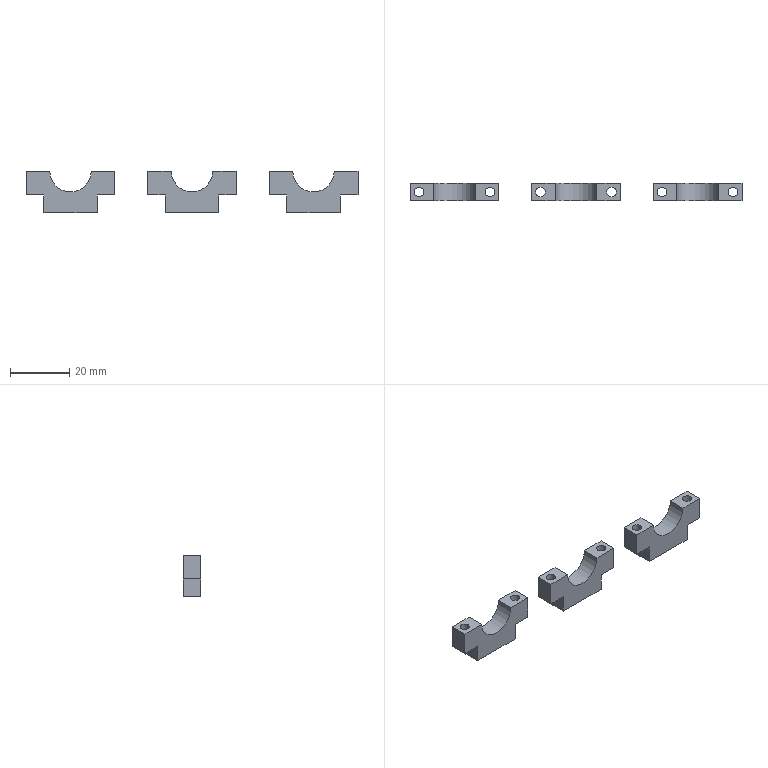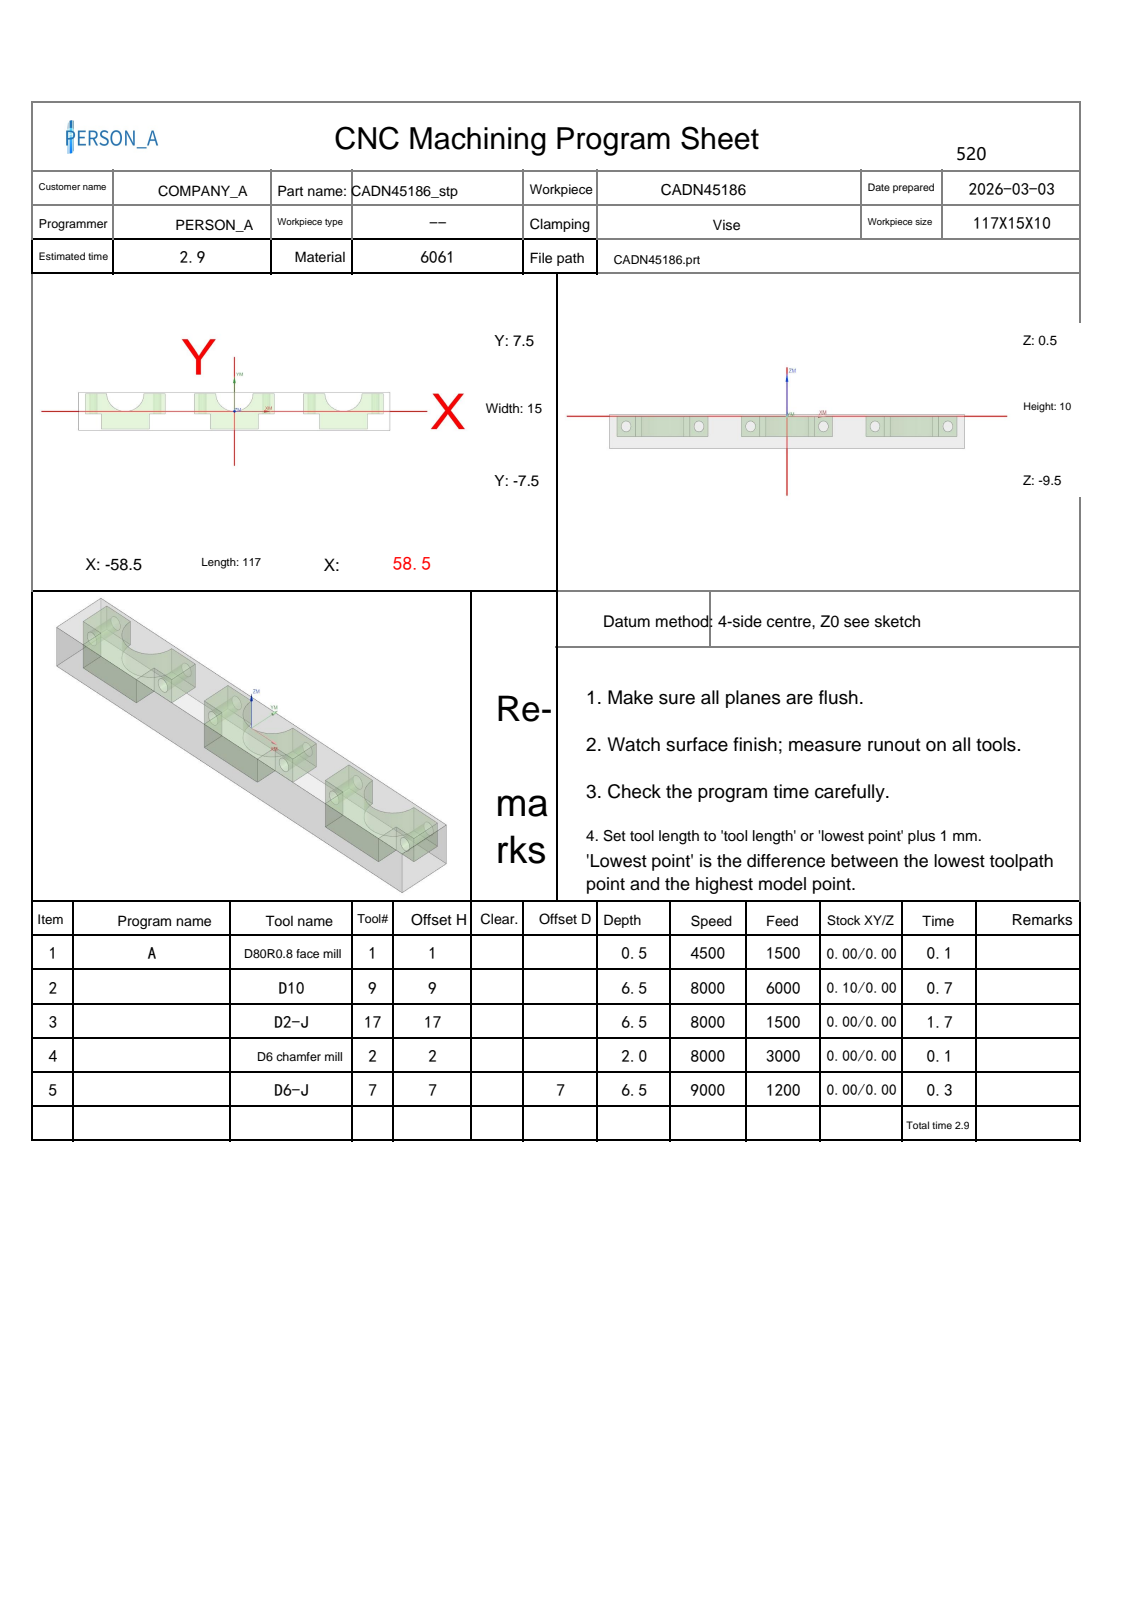NC program | NX | posted by the shop | part box 112 x 6 x 14 mm
Lines 634 to 1728 of 5059:
N3 T17 M06
(D2-J  D=2. R=0. H=17 ce=0.00 di=0.00)
(MAX_Z=50. MIN_Z=-6. Time=1.66M)
G00 G90 G54 X55.15 Y-2.2 M03 S8000
G43 H17 Z50.
M08
Z0.0
G01 X55.149 Y-2.197 Z-.03 F1500.
X55.147 Y-2.19 Z-.058
X55.144 Y-2.179 Z-.082
X55.139 Y-2.165 Z-.104
X55.133 Y-2.148 Z-.123
X55.125 Y-2.13 Z-.14
X55.115 Y-2.11 Z-.154
X55.103 Y-2.09 Z-.166
X55.089 Y-2.07 Z-.176
X55.072 Y-2.052 Z-.184
X55.053 Y-2.035 Z-.19
X55.032 Y-2.021 Z-.195
X55.007 Y-2.01 Z-.198
X54.98 Y-2.003 Z-.199
X54.95 Y-2. Z-.2
X51.
Y-5.95
X51.014 Y-5.964 Z-.201
X51.056 Y-5.953 Z-.202
X51.121 Y-5.919 Z-.205
X51.209 Y-5.864 Z-.209
X51.565 Y-5.599 Z-.225
X51.878 Y-5.345 Z-.239
X52.111 Y-5.146 Z-.249
X52.375 Y-4.909 Z-.262
X52.674 Y-4.632 Z-.276
X52.995 Y-4.322 Z-.292
X53.322 Y-3.995 Z-.308
X53.632 Y-3.674 Z-.324
X53.909 Y-3.375 Z-.338
X54.146 Y-3.111 Z-.351
X54.345 Y-2.878 Z-.361
X54.599 Y-2.565 Z-.375
X54.864 Y-2.209 Z-.391
X54.919 Y-2.121 Z-.395
X54.953 Y-2.056 Z-.398
X54.964 Y-2.014 Z-.399
X54.95 Y-2. Z-.4
X51.
Y-5.95
X51.014 Y-5.964 Z-.401
X51.056 Y-5.953 Z-.402
X51.121 Y-5.919 Z-.405
X51.209 Y-5.864 Z-.409
X51.565 Y-5.599 Z-.425
X51.878 Y-5.345 Z-.439
X52.111 Y-5.146 Z-.449
X52.375 Y-4.909 Z-.462
X52.674 Y-4.632 Z-.476
X52.995 Y-4.322 Z-.492
X53.322 Y-3.995 Z-.508
X53.632 Y-3.674 Z-.524
X53.909 Y-3.375 Z-.538
X54.146 Y-3.111 Z-.551
X54.345 Y-2.878 Z-.561
X54.599 Y-2.565 Z-.575
X54.864 Y-2.209 Z-.591
X54.919 Y-2.121 Z-.595
X54.953 Y-2.056 Z-.598
X54.964 Y-2.014 Z-.599
X54.95 Y-2. Z-.6
X51.
Y-5.95
X51.014 Y-5.964 Z-.601
X51.056 Y-5.953 Z-.602
X51.121 Y-5.919 Z-.605
X51.209 Y-5.864 Z-.609
X51.565 Y-5.599 Z-.625
X51.878 Y-5.345 Z-.639
X52.111 Y-5.146 Z-.649
X52.375 Y-4.909 Z-.662
X52.674 Y-4.632 Z-.676
X52.995 Y-4.322 Z-.692
X53.322 Y-3.995 Z-.708
X53.632 Y-3.674 Z-.724
X53.909 Y-3.375 Z-.738
X54.146 Y-3.111 Z-.751
X54.345 Y-2.878 Z-.761
X54.599 Y-2.565 Z-.775
X54.864 Y-2.209 Z-.791
X54.919 Y-2.121 Z-.795
X54.953 Y-2.056 Z-.798
X54.964 Y-2.014 Z-.799
X54.95 Y-2. Z-.8
X51.
Y-5.95
X51.014 Y-5.964 Z-.801
X51.056 Y-5.953 Z-.802
X51.121 Y-5.919 Z-.805
X51.209 Y-5.864 Z-.809
X51.565 Y-5.599 Z-.825
X51.878 Y-5.345 Z-.839
X52.111 Y-5.146 Z-.849
X52.375 Y-4.909 Z-.862
X52.674 Y-4.632 Z-.876
X52.995 Y-4.322 Z-.892
X53.322 Y-3.995 Z-.908
X53.632 Y-3.674 Z-.924
X53.909 Y-3.375 Z-.938
X54.146 Y-3.111 Z-.951
X54.345 Y-2.878 Z-.961
X54.599 Y-2.565 Z-.975
X54.864 Y-2.209 Z-.991
X54.919 Y-2.121 Z-.995
X54.953 Y-2.056 Z-.998
X54.964 Y-2.014 Z-.999
X54.95 Y-2. Z-1.
X51.
Y-5.95
X51.014 Y-5.964 Z-1.001
X51.056 Y-5.953 Z-1.002
X51.121 Y-5.919 Z-1.005
X51.209 Y-5.864 Z-1.009
X51.565 Y-5.599 Z-1.025
X51.878 Y-5.345 Z-1.039
X52.111 Y-5.146 Z-1.049
X52.375 Y-4.909 Z-1.062
X52.674 Y-4.632 Z-1.076
X52.995 Y-4.322 Z-1.092
X53.322 Y-3.995 Z-1.108
X53.632 Y-3.674 Z-1.124
X53.909 Y-3.375 Z-1.138
X54.146 Y-3.111 Z-1.151
X54.345 Y-2.878 Z-1.161
X54.599 Y-2.565 Z-1.175
X54.864 Y-2.209 Z-1.191
X54.919 Y-2.121 Z-1.195
X54.953 Y-2.056 Z-1.198
X54.964 Y-2.014 Z-1.199
X54.95 Y-2. Z-1.2
X51.
Y-5.95
X51.014 Y-5.964 Z-1.201
X51.056 Y-5.953 Z-1.202
X51.121 Y-5.919 Z-1.205
X51.209 Y-5.864 Z-1.209
X51.565 Y-5.599 Z-1.225
X51.878 Y-5.345 Z-1.239
X52.111 Y-5.146 Z-1.249
X52.375 Y-4.909 Z-1.262
X52.674 Y-4.632 Z-1.276
X52.995 Y-4.322 Z-1.292
X53.322 Y-3.995 Z-1.308
X53.632 Y-3.674 Z-1.324
X53.909 Y-3.375 Z-1.338
X54.146 Y-3.111 Z-1.351
X54.345 Y-2.878 Z-1.361
X54.599 Y-2.565 Z-1.375
X54.864 Y-2.209 Z-1.391
X54.919 Y-2.121 Z-1.395
X54.953 Y-2.056 Z-1.398
X54.964 Y-2.014 Z-1.399
X54.95 Y-2. Z-1.4
X51.
Y-5.95
X51.014 Y-5.964 Z-1.401
X51.056 Y-5.953 Z-1.402
X51.121 Y-5.919 Z-1.405
X51.209 Y-5.864 Z-1.409
X51.565 Y-5.599 Z-1.425
X51.878 Y-5.345 Z-1.439
X52.111 Y-5.146 Z-1.449
X52.375 Y-4.909 Z-1.462
X52.674 Y-4.632 Z-1.476
X52.995 Y-4.322 Z-1.492
X53.322 Y-3.995 Z-1.508
X53.632 Y-3.674 Z-1.524
X53.909 Y-3.375 Z-1.538
X54.146 Y-3.111 Z-1.551
X54.345 Y-2.878 Z-1.561
X54.599 Y-2.565 Z-1.575
X54.864 Y-2.209 Z-1.591
X54.919 Y-2.121 Z-1.595
X54.953 Y-2.056 Z-1.598
X54.964 Y-2.014 Z-1.599
X54.95 Y-2. Z-1.6
X51.
Y-5.95
X51.014 Y-5.964 Z-1.601
X51.056 Y-5.953 Z-1.602
X51.121 Y-5.919 Z-1.605
X51.209 Y-5.864 Z-1.609
X51.565 Y-5.599 Z-1.625
X51.878 Y-5.345 Z-1.639
X52.111 Y-5.146 Z-1.649
X52.375 Y-4.909 Z-1.662
X52.674 Y-4.632 Z-1.676
X52.995 Y-4.322 Z-1.692
X53.322 Y-3.995 Z-1.708
X53.632 Y-3.674 Z-1.724
X53.909 Y-3.375 Z-1.738
X54.146 Y-3.111 Z-1.751
X54.345 Y-2.878 Z-1.761
X54.599 Y-2.565 Z-1.775
X54.864 Y-2.209 Z-1.791
X54.919 Y-2.121 Z-1.795
X54.953 Y-2.056 Z-1.798
X54.964 Y-2.014 Z-1.799
X54.95 Y-2. Z-1.8
X51.
Y-5.95
X51.014 Y-5.964 Z-1.801
X51.056 Y-5.953 Z-1.802
X51.121 Y-5.919 Z-1.805
X51.209 Y-5.864 Z-1.809
X51.565 Y-5.599 Z-1.825
X51.878 Y-5.345 Z-1.839
X52.111 Y-5.146 Z-1.849
X52.375 Y-4.909 Z-1.862
X52.674 Y-4.632 Z-1.876
X52.995 Y-4.322 Z-1.892
X53.322 Y-3.995 Z-1.908
X53.632 Y-3.674 Z-1.924
X53.909 Y-3.375 Z-1.938
X54.146 Y-3.111 Z-1.951
X54.345 Y-2.878 Z-1.961
X54.599 Y-2.565 Z-1.975
X54.864 Y-2.209 Z-1.991
X54.919 Y-2.121 Z-1.995
X54.953 Y-2.056 Z-1.998
X54.964 Y-2.014 Z-1.999
X54.95 Y-2. Z-2.
X51.
Y-5.95
X51.014 Y-5.964 Z-2.001
X51.056 Y-5.953 Z-2.002
X51.121 Y-5.919 Z-2.005
X51.209 Y-5.864 Z-2.009
X51.565 Y-5.599 Z-2.025
X51.878 Y-5.345 Z-2.039
X52.111 Y-5.146 Z-2.049
X52.375 Y-4.909 Z-2.062
X52.674 Y-4.632 Z-2.076
X52.995 Y-4.322 Z-2.092
X53.322 Y-3.995 Z-2.108
X53.632 Y-3.674 Z-2.124
X53.909 Y-3.375 Z-2.138
X54.146 Y-3.111 Z-2.151
X54.345 Y-2.878 Z-2.161
X54.599 Y-2.565 Z-2.175
X54.864 Y-2.209 Z-2.191
X54.919 Y-2.121 Z-2.195
X54.953 Y-2.056 Z-2.198
X54.964 Y-2.014 Z-2.199
X54.95 Y-2. Z-2.2
X51.
Y-5.95
X51.014 Y-5.964 Z-2.201
X51.056 Y-5.953 Z-2.202
X51.121 Y-5.919 Z-2.205
X51.209 Y-5.864 Z-2.209
X51.565 Y-5.599 Z-2.225
X51.878 Y-5.345 Z-2.239
X52.111 Y-5.146 Z-2.249
X52.375 Y-4.909 Z-2.262
X52.674 Y-4.632 Z-2.276
X52.995 Y-4.322 Z-2.292
X53.322 Y-3.995 Z-2.308
X53.632 Y-3.674 Z-2.324
X53.909 Y-3.375 Z-2.338
X54.146 Y-3.111 Z-2.351
X54.345 Y-2.878 Z-2.361
X54.599 Y-2.565 Z-2.375
X54.864 Y-2.209 Z-2.391
X54.919 Y-2.121 Z-2.395
X54.953 Y-2.056 Z-2.398
X54.964 Y-2.014 Z-2.399
X54.95 Y-2. Z-2.4
X51.
Y-5.95
X51.014 Y-5.964 Z-2.401
X51.056 Y-5.953 Z-2.402
X51.121 Y-5.919 Z-2.405
X51.209 Y-5.864 Z-2.409
X51.565 Y-5.599 Z-2.425
X51.878 Y-5.345 Z-2.439
X52.111 Y-5.146 Z-2.449
X52.375 Y-4.909 Z-2.462
X52.674 Y-4.632 Z-2.476
X52.995 Y-4.322 Z-2.492
X53.322 Y-3.995 Z-2.508
X53.632 Y-3.674 Z-2.524
X53.909 Y-3.375 Z-2.538
X54.146 Y-3.111 Z-2.551
X54.345 Y-2.878 Z-2.561
X54.599 Y-2.565 Z-2.575
X54.864 Y-2.209 Z-2.591
X54.919 Y-2.121 Z-2.595
X54.953 Y-2.056 Z-2.598
X54.964 Y-2.014 Z-2.599
X54.95 Y-2. Z-2.6
X51.
Y-5.95
X51.014 Y-5.964 Z-2.601
X51.056 Y-5.953 Z-2.602
X51.121 Y-5.919 Z-2.605
X51.209 Y-5.864 Z-2.609
X51.565 Y-5.599 Z-2.625
X51.878 Y-5.345 Z-2.639
X52.111 Y-5.146 Z-2.649
X52.375 Y-4.909 Z-2.662
X52.674 Y-4.632 Z-2.676
X52.995 Y-4.322 Z-2.692
X53.322 Y-3.995 Z-2.708
X53.632 Y-3.674 Z-2.724
X53.909 Y-3.375 Z-2.738
X54.146 Y-3.111 Z-2.751
X54.345 Y-2.878 Z-2.761
X54.599 Y-2.565 Z-2.775
X54.864 Y-2.209 Z-2.791
X54.919 Y-2.121 Z-2.795
X54.953 Y-2.056 Z-2.798
X54.964 Y-2.014 Z-2.799
X54.95 Y-2. Z-2.8
X51.
Y-5.95
X51.014 Y-5.964 Z-2.801
X51.056 Y-5.953 Z-2.802
X51.121 Y-5.919 Z-2.805
X51.209 Y-5.864 Z-2.809
X51.565 Y-5.599 Z-2.825
X51.878 Y-5.345 Z-2.839
X52.111 Y-5.146 Z-2.849
X52.375 Y-4.909 Z-2.862
X52.674 Y-4.632 Z-2.876
X52.995 Y-4.322 Z-2.892
X53.322 Y-3.995 Z-2.908
X53.632 Y-3.674 Z-2.924
X53.909 Y-3.375 Z-2.938
X54.146 Y-3.111 Z-2.951
X54.345 Y-2.878 Z-2.961
X54.599 Y-2.565 Z-2.975
X54.864 Y-2.209 Z-2.991
X54.919 Y-2.121 Z-2.995
X54.953 Y-2.056 Z-2.998
X54.964 Y-2.014 Z-2.999
X54.95 Y-2. Z-3.
X51.
Y-5.95
X51.014 Y-5.964 Z-3.001
X51.056 Y-5.953 Z-3.002
X51.121 Y-5.919 Z-3.005
X51.209 Y-5.864 Z-3.009
X51.565 Y-5.599 Z-3.025
X51.878 Y-5.345 Z-3.039
X52.111 Y-5.146 Z-3.049
X52.375 Y-4.909 Z-3.062
X52.674 Y-4.632 Z-3.076
X52.995 Y-4.322 Z-3.092
X53.322 Y-3.995 Z-3.108
X53.632 Y-3.674 Z-3.124
X53.909 Y-3.375 Z-3.138
X54.146 Y-3.111 Z-3.151
X54.345 Y-2.878 Z-3.161
X54.599 Y-2.565 Z-3.175
X54.864 Y-2.209 Z-3.191
X54.919 Y-2.121 Z-3.195
X54.953 Y-2.056 Z-3.198
X54.964 Y-2.014 Z-3.199
X54.95 Y-2. Z-3.2
X51.
Y-5.95
X51.014 Y-5.964 Z-3.201
X51.056 Y-5.953 Z-3.202
X51.121 Y-5.919 Z-3.205
X51.209 Y-5.864 Z-3.209
X51.565 Y-5.599 Z-3.225
X51.878 Y-5.345 Z-3.239
X52.111 Y-5.146 Z-3.249
X52.375 Y-4.909 Z-3.262
X52.674 Y-4.632 Z-3.276
X52.995 Y-4.322 Z-3.292
X53.322 Y-3.995 Z-3.308
X53.632 Y-3.674 Z-3.324
X53.909 Y-3.375 Z-3.338
X54.146 Y-3.111 Z-3.351
X54.345 Y-2.878 Z-3.361
X54.599 Y-2.565 Z-3.375
X54.864 Y-2.209 Z-3.391
X54.919 Y-2.121 Z-3.395
X54.953 Y-2.056 Z-3.398
X54.964 Y-2.014 Z-3.399
X54.95 Y-2. Z-3.4
X51.
Y-5.95
X51.014 Y-5.964 Z-3.401
X51.056 Y-5.953 Z-3.402
X51.121 Y-5.919 Z-3.405
X51.209 Y-5.864 Z-3.409
X51.565 Y-5.599 Z-3.425
X51.878 Y-5.345 Z-3.439
X52.111 Y-5.146 Z-3.449
X52.375 Y-4.909 Z-3.462
X52.674 Y-4.632 Z-3.476
X52.995 Y-4.322 Z-3.492
X53.322 Y-3.995 Z-3.508
X53.632 Y-3.674 Z-3.524
X53.909 Y-3.375 Z-3.538
X54.146 Y-3.111 Z-3.551
X54.345 Y-2.878 Z-3.561
X54.599 Y-2.565 Z-3.575
X54.864 Y-2.209 Z-3.591
X54.919 Y-2.121 Z-3.595
X54.953 Y-2.056 Z-3.598
X54.964 Y-2.014 Z-3.599
X54.95 Y-2. Z-3.6
X51.
Y-5.95
X51.014 Y-5.964 Z-3.601
X51.056 Y-5.953 Z-3.602
X51.121 Y-5.919 Z-3.605
X51.209 Y-5.864 Z-3.609
X51.565 Y-5.599 Z-3.625
X51.878 Y-5.345 Z-3.639
X52.111 Y-5.146 Z-3.649
X52.375 Y-4.909 Z-3.662
X52.674 Y-4.632 Z-3.676
X52.995 Y-4.322 Z-3.692
X53.322 Y-3.995 Z-3.708
X53.632 Y-3.674 Z-3.724
X53.909 Y-3.375 Z-3.738
X54.146 Y-3.111 Z-3.751
X54.345 Y-2.878 Z-3.761
X54.599 Y-2.565 Z-3.775
X54.864 Y-2.209 Z-3.791
X54.919 Y-2.121 Z-3.795
X54.953 Y-2.056 Z-3.798
X54.964 Y-2.014 Z-3.799
X54.95 Y-2. Z-3.8
X51.
Y-5.95
X51.014 Y-5.964 Z-3.801
X51.056 Y-5.953 Z-3.802
X51.121 Y-5.919 Z-3.805
X51.209 Y-5.864 Z-3.809
X51.565 Y-5.599 Z-3.825
X51.878 Y-5.345 Z-3.839
X52.111 Y-5.146 Z-3.849
X52.375 Y-4.909 Z-3.862
X52.674 Y-4.632 Z-3.876
X52.995 Y-4.322 Z-3.892
X53.322 Y-3.995 Z-3.908
X53.632 Y-3.674 Z-3.924
X53.909 Y-3.375 Z-3.938
X54.146 Y-3.111 Z-3.951
X54.345 Y-2.878 Z-3.961
X54.599 Y-2.565 Z-3.975
X54.864 Y-2.209 Z-3.991
X54.919 Y-2.121 Z-3.995
X54.953 Y-2.056 Z-3.998
X54.964 Y-2.014 Z-3.999
X54.95 Y-2. Z-4.
X51.
Y-5.95
X51.014 Y-5.964 Z-4.001
X51.056 Y-5.953 Z-4.002
X51.121 Y-5.919 Z-4.005
X51.209 Y-5.864 Z-4.009
X51.565 Y-5.599 Z-4.025
X51.878 Y-5.345 Z-4.039
X52.111 Y-5.146 Z-4.049
X52.375 Y-4.909 Z-4.062
X52.674 Y-4.632 Z-4.076
X52.995 Y-4.322 Z-4.092
X53.322 Y-3.995 Z-4.108
X53.632 Y-3.674 Z-4.124
X53.909 Y-3.375 Z-4.138
X54.146 Y-3.111 Z-4.151
X54.345 Y-2.878 Z-4.161
X54.599 Y-2.565 Z-4.175
X54.864 Y-2.209 Z-4.191
X54.919 Y-2.121 Z-4.195
X54.953 Y-2.056 Z-4.198
X54.964 Y-2.014 Z-4.199
X54.95 Y-2. Z-4.2
X51.
Y-5.95
X51.014 Y-5.964 Z-4.201
X51.056 Y-5.953 Z-4.202
X51.121 Y-5.919 Z-4.205
X51.209 Y-5.864 Z-4.209
X51.565 Y-5.599 Z-4.225
X51.878 Y-5.345 Z-4.239
X52.111 Y-5.146 Z-4.249
X52.375 Y-4.909 Z-4.262
X52.674 Y-4.632 Z-4.276
X52.995 Y-4.322 Z-4.292
X53.322 Y-3.995 Z-4.308
X53.632 Y-3.674 Z-4.324
X53.909 Y-3.375 Z-4.338
X54.146 Y-3.111 Z-4.351
X54.345 Y-2.878 Z-4.361
X54.599 Y-2.565 Z-4.375
X54.864 Y-2.209 Z-4.391
X54.919 Y-2.121 Z-4.395
X54.953 Y-2.056 Z-4.398
X54.964 Y-2.014 Z-4.399
X54.95 Y-2. Z-4.4
X51.
Y-5.95
X51.014 Y-5.964 Z-4.401
X51.056 Y-5.953 Z-4.402
X51.121 Y-5.919 Z-4.405
X51.209 Y-5.864 Z-4.409
X51.565 Y-5.599 Z-4.425
X51.878 Y-5.345 Z-4.439
X52.111 Y-5.146 Z-4.449
X52.375 Y-4.909 Z-4.462
X52.674 Y-4.632 Z-4.476
X52.995 Y-4.322 Z-4.492
X53.322 Y-3.995 Z-4.508
X53.632 Y-3.674 Z-4.524
X53.909 Y-3.375 Z-4.538
X54.146 Y-3.111 Z-4.551
X54.345 Y-2.878 Z-4.561
X54.599 Y-2.565 Z-4.575
X54.864 Y-2.209 Z-4.591
X54.919 Y-2.121 Z-4.595
X54.953 Y-2.056 Z-4.598
X54.964 Y-2.014 Z-4.599
X54.95 Y-2. Z-4.6
X51.
Y-5.95
X51.014 Y-5.964 Z-4.601
X51.056 Y-5.953 Z-4.602
X51.121 Y-5.919 Z-4.605
X51.209 Y-5.864 Z-4.609
X51.565 Y-5.599 Z-4.625
X51.878 Y-5.345 Z-4.639
X52.111 Y-5.146 Z-4.649
X52.375 Y-4.909 Z-4.662
X52.674 Y-4.632 Z-4.676
X52.995 Y-4.322 Z-4.692
X53.322 Y-3.995 Z-4.708
X53.632 Y-3.674 Z-4.724
X53.909 Y-3.375 Z-4.738
X54.146 Y-3.111 Z-4.751
X54.345 Y-2.878 Z-4.761
X54.599 Y-2.565 Z-4.775
X54.864 Y-2.209 Z-4.791
X54.919 Y-2.121 Z-4.795
X54.953 Y-2.056 Z-4.798
X54.964 Y-2.014 Z-4.799
X54.95 Y-2. Z-4.8
X51.
Y-5.95
X51.014 Y-5.964 Z-4.801
X51.056 Y-5.953 Z-4.802
X51.121 Y-5.919 Z-4.805
X51.209 Y-5.864 Z-4.809
X51.565 Y-5.599 Z-4.825
X51.878 Y-5.345 Z-4.839
X52.111 Y-5.146 Z-4.849
X52.375 Y-4.909 Z-4.862
X52.674 Y-4.632 Z-4.876
X52.995 Y-4.322 Z-4.892
X53.322 Y-3.995 Z-4.908
X53.632 Y-3.674 Z-4.924
X53.909 Y-3.375 Z-4.938
X54.146 Y-3.111 Z-4.951
X54.345 Y-2.878 Z-4.961
X54.599 Y-2.565 Z-4.975
X54.864 Y-2.209 Z-4.991
X54.919 Y-2.121 Z-4.995
X54.953 Y-2.056 Z-4.998
X54.964 Y-2.014 Z-4.999
X54.95 Y-2. Z-5.
X51.
Y-5.95
X51.014 Y-5.964 Z-5.001
X51.056 Y-5.953 Z-5.002
X51.121 Y-5.919 Z-5.005
X51.209 Y-5.864 Z-5.009
X51.565 Y-5.599 Z-5.025
X51.878 Y-5.345 Z-5.039
X52.111 Y-5.146 Z-5.049
X52.375 Y-4.909 Z-5.062
X52.674 Y-4.632 Z-5.076
X52.995 Y-4.322 Z-5.092
X53.322 Y-3.995 Z-5.108
X53.632 Y-3.674 Z-5.124
X53.909 Y-3.375 Z-5.138
X54.146 Y-3.111 Z-5.151
X54.345 Y-2.878 Z-5.161
X54.599 Y-2.565 Z-5.175
X54.864 Y-2.209 Z-5.191
X54.919 Y-2.121 Z-5.195
X54.953 Y-2.056 Z-5.198
X54.964 Y-2.014 Z-5.199
X54.95 Y-2. Z-5.2
X51.
Y-5.95
X51.014 Y-5.964 Z-5.201
X51.056 Y-5.953 Z-5.202
X51.121 Y-5.919 Z-5.205
X51.209 Y-5.864 Z-5.209
X51.565 Y-5.599 Z-5.225
X51.878 Y-5.345 Z-5.239
X52.111 Y-5.146 Z-5.249
X52.375 Y-4.909 Z-5.262
X52.674 Y-4.632 Z-5.276
X52.995 Y-4.322 Z-5.292
X53.322 Y-3.995 Z-5.308
X53.632 Y-3.674 Z-5.324
X53.909 Y-3.375 Z-5.338
X54.146 Y-3.111 Z-5.351
X54.345 Y-2.878 Z-5.361
X54.599 Y-2.565 Z-5.375
X54.864 Y-2.209 Z-5.391
X54.919 Y-2.121 Z-5.395
X54.953 Y-2.056 Z-5.398
X54.964 Y-2.014 Z-5.399
X54.95 Y-2. Z-5.4
X51.
Y-5.95
X51.014 Y-5.964 Z-5.401
X51.056 Y-5.953 Z-5.402
X51.121 Y-5.919 Z-5.405
X51.209 Y-5.864 Z-5.409
X51.565 Y-5.599 Z-5.425
X51.878 Y-5.345 Z-5.439
X52.111 Y-5.146 Z-5.449
X52.375 Y-4.909 Z-5.462
X52.674 Y-4.632 Z-5.476
X52.995 Y-4.322 Z-5.492
X53.322 Y-3.995 Z-5.508
X53.632 Y-3.674 Z-5.524
X53.909 Y-3.375 Z-5.538
X54.146 Y-3.111 Z-5.551
X54.345 Y-2.878 Z-5.561
X54.599 Y-2.565 Z-5.575
X54.864 Y-2.209 Z-5.591
X54.919 Y-2.121 Z-5.595
X54.953 Y-2.056 Z-5.598
X54.964 Y-2.014 Z-5.599
X54.95 Y-2. Z-5.6
X51.
Y-5.95
X51.014 Y-5.964 Z-5.601
X51.056 Y-5.953 Z-5.602
X51.121 Y-5.919 Z-5.605
X51.209 Y-5.864 Z-5.609
X51.565 Y-5.599 Z-5.625
X51.878 Y-5.345 Z-5.639
X52.111 Y-5.146 Z-5.649
X52.375 Y-4.909 Z-5.662
X52.674 Y-4.632 Z-5.676
X52.995 Y-4.322 Z-5.692
X53.322 Y-3.995 Z-5.708
X53.632 Y-3.674 Z-5.724
X53.909 Y-3.375 Z-5.738
X54.146 Y-3.111 Z-5.751
X54.345 Y-2.878 Z-5.761
X54.599 Y-2.565 Z-5.775
X54.864 Y-2.209 Z-5.791
X54.919 Y-2.121 Z-5.795
X54.953 Y-2.056 Z-5.798
X54.964 Y-2.014 Z-5.799
X54.95 Y-2. Z-5.8
X51.
Y-5.95
X51.014 Y-5.964 Z-5.801
X51.056 Y-5.953 Z-5.802
X51.121 Y-5.919 Z-5.805
X51.209 Y-5.864 Z-5.809
X51.565 Y-5.599 Z-5.825
X51.878 Y-5.345 Z-5.839
X52.111 Y-5.146 Z-5.849
X52.375 Y-4.909 Z-5.862
X52.674 Y-4.632 Z-5.876
X52.995 Y-4.322 Z-5.892
X53.322 Y-3.995 Z-5.908
X53.632 Y-3.674 Z-5.924
X53.909 Y-3.375 Z-5.938
X54.146 Y-3.111 Z-5.951
X54.345 Y-2.878 Z-5.961
X54.599 Y-2.565 Z-5.975
X54.864 Y-2.209 Z-5.991
X54.919 Y-2.121 Z-5.995
X54.953 Y-2.056 Z-5.998
X54.964 Y-2.014 Z-5.999
X54.95 Y-2. Z-6.
X51.
Y-5.95
X51.003 Y-5.98 Z-5.999
X51.01 Y-6.007 Z-5.998
X51.021 Y-6.032 Z-5.995
X51.035 Y-6.053 Z-5.99
X51.052 Y-6.072 Z-5.984
X51.07 Y-6.089 Z-5.976
X51.09 Y-6.103 Z-5.966
X51.11 Y-6.115 Z-5.954
X51.13 Y-6.125 Z-5.94
X51.148 Y-6.133 Z-5.923
X51.165 Y-6.139 Z-5.904
X51.179 Y-6.144 Z-5.882
X51.19 Y-6.147 Z-5.858
X51.197 Y-6.149 Z-5.83
X51.2 Y-6.15 Z-5.8
G00 Z50.
X30.799 Y-6.153
Z0.0
G01 X30.802 Z-.03
X30.809 Y-6.151 Z-.058
X30.82 Y-6.147 Z-.082
X30.834 Y-6.143 Z-.104
X30.851 Y-6.136 Z-.123
X30.87 Y-6.128 Z-.14
X30.89 Y-6.117 Z-.154
X30.91 Y-6.105 Z-.166
X30.929 Y-6.09 Z-.176
X30.948 Y-6.073 Z-.184
X30.965 Y-6.054 Z-.19
X30.979 Y-6.032 Z-.195
X30.99 Y-6.007 Z-.198
X30.997 Y-5.98 Z-.199
X31. Y-5.95 Z-.2
Y-2.
X27.051
X27.036 Y-2.014 Z-.201
X27.047 Y-2.056 Z-.202
X27.081 Y-2.121 Z-.205
X27.136 Y-2.209 Z-.209
X27.401 Y-2.566 Z-.225
X27.655 Y-2.878 Z-.239
X27.854 Y-3.111 Z-.249
X28.091 Y-3.376 Z-.262
X28.368 Y-3.675 Z-.276
X28.678 Y-3.997 Z-.292
X29.004 Y-4.323 Z-.308
X29.326 Y-4.633 Z-.324
X29.624 Y-4.911 Z-.338
X29.889 Y-5.147 Z-.351
X30.122 Y-5.347 Z-.361
X30.434 Y-5.6 Z-.375
X30.791 Y-5.864 Z-.391
X30.879 Y-5.919 Z-.395
X30.944 Y-5.953 Z-.398
X30.986 Y-5.964 Z-.399
X31. Y-5.95 Z-.4
Y-2.
X27.051
X27.036 Y-2.014 Z-.401
X27.047 Y-2.056 Z-.402
X27.081 Y-2.121 Z-.405
X27.136 Y-2.209 Z-.409
X27.401 Y-2.566 Z-.425
X27.655 Y-2.878 Z-.439
X27.854 Y-3.111 Z-.449
X28.091 Y-3.376 Z-.462
X28.368 Y-3.675 Z-.476
X28.678 Y-3.997 Z-.492
X29.004 Y-4.323 Z-.508
X29.326 Y-4.633 Z-.524
X29.624 Y-4.911 Z-.538
X29.889 Y-5.147 Z-.551
X30.122 Y-5.347 Z-.561
X30.434 Y-5.6 Z-.575
X30.791 Y-5.864 Z-.591
X30.879 Y-5.919 Z-.595
X30.944 Y-5.953 Z-.598
X30.986 Y-5.964 Z-.599
X31. Y-5.95 Z-.6
Y-2.
X27.051
X27.036 Y-2.014 Z-.601
X27.047 Y-2.056 Z-.602
X27.081 Y-2.121 Z-.605
X27.136 Y-2.209 Z-.609
X27.401 Y-2.566 Z-.625
X27.655 Y-2.878 Z-.639
X27.854 Y-3.111 Z-.649
X28.091 Y-3.376 Z-.662
X28.368 Y-3.675 Z-.676
X28.678 Y-3.997 Z-.692
X29.004 Y-4.323 Z-.708
X29.326 Y-4.633 Z-.724
X29.624 Y-4.911 Z-.738
X29.889 Y-5.147 Z-.751
X30.122 Y-5.347 Z-.761
X30.434 Y-5.6 Z-.775
X30.791 Y-5.864 Z-.791
X30.879 Y-5.919 Z-.795
X30.944 Y-5.953 Z-.798
X30.986 Y-5.964 Z-.799
X31. Y-5.95 Z-.8
Y-2.
X27.051
X27.036 Y-2.014 Z-.801
X27.047 Y-2.056 Z-.802
X27.081 Y-2.121 Z-.805
X27.136 Y-2.209 Z-.809
X27.401 Y-2.566 Z-.825
X27.655 Y-2.878 Z-.839
X27.854 Y-3.111 Z-.849
X28.091 Y-3.376 Z-.862
X28.368 Y-3.675 Z-.876
X28.678 Y-3.997 Z-.892
X29.004 Y-4.323 Z-.908
X29.326 Y-4.633 Z-.924
X29.624 Y-4.911 Z-.938
X29.889 Y-5.147 Z-.951
X30.122 Y-5.347 Z-.961
X30.434 Y-5.6 Z-.975
X30.791 Y-5.864 Z-.991
X30.879 Y-5.919 Z-.995
X30.944 Y-5.953 Z-.998
X30.986 Y-5.964 Z-.999
X31. Y-5.95 Z-1.
Y-2.
X27.051
X27.036 Y-2.014 Z-1.001
X27.047 Y-2.056 Z-1.002
X27.081 Y-2.121 Z-1.005
X27.136 Y-2.209 Z-1.009
X27.401 Y-2.566 Z-1.025
X27.655 Y-2.878 Z-1.039
X27.854 Y-3.111 Z-1.049
X28.091 Y-3.376 Z-1.062
X28.368 Y-3.675 Z-1.076
X28.678 Y-3.997 Z-1.092
X29.004 Y-4.323 Z-1.108
X29.326 Y-4.633 Z-1.124
X29.624 Y-4.911 Z-1.138
X29.889 Y-5.147 Z-1.151
X30.122 Y-5.347 Z-1.161
X30.434 Y-5.6 Z-1.175
X30.791 Y-5.864 Z-1.191
X30.879 Y-5.919 Z-1.195
X30.944 Y-5.953 Z-1.198
X30.986 Y-5.964 Z-1.199
X31. Y-5.95 Z-1.2
Y-2.
X27.051
X27.036 Y-2.014 Z-1.201
X27.047 Y-2.056 Z-1.202
X27.081 Y-2.121 Z-1.205
X27.136 Y-2.209 Z-1.209
X27.401 Y-2.566 Z-1.225
X27.655 Y-2.878 Z-1.239
X27.854 Y-3.111 Z-1.249
X28.091 Y-3.376 Z-1.262
X28.368 Y-3.675 Z-1.276
X28.678 Y-3.997 Z-1.292
X29.004 Y-4.323 Z-1.308
X29.326 Y-4.633 Z-1.324
X29.624 Y-4.911 Z-1.338
X29.889 Y-5.147 Z-1.351
X30.122 Y-5.347 Z-1.361
X30.434 Y-5.6 Z-1.375
X30.791 Y-5.864 Z-1.391
X30.879 Y-5.919 Z-1.395
X30.944 Y-5.953 Z-1.398
X30.986 Y-5.964 Z-1.399
X31. Y-5.95 Z-1.4
Y-2.
X27.051
X27.036 Y-2.014 Z-1.401
X27.047 Y-2.056 Z-1.402
X27.081 Y-2.121 Z-1.405
X27.136 Y-2.209 Z-1.409
X27.401 Y-2.566 Z-1.425
X27.655 Y-2.878 Z-1.439
X27.854 Y-3.111 Z-1.449
X28.091 Y-3.376 Z-1.462
X28.368 Y-3.675 Z-1.476
X28.678 Y-3.997 Z-1.492
X29.004 Y-4.323 Z-1.508
X29.326 Y-4.633 Z-1.524
X29.624 Y-4.911 Z-1.538
X29.889 Y-5.147 Z-1.551
X30.122 Y-5.347 Z-1.561
X30.434 Y-5.6 Z-1.575
X30.791 Y-5.864 Z-1.591
X30.879 Y-5.919 Z-1.595
X30.944 Y-5.953 Z-1.598
X30.986 Y-5.964 Z-1.599
X31. Y-5.95 Z-1.6
Y-2.
X27.051
X27.036 Y-2.014 Z-1.601
X27.047 Y-2.056 Z-1.602
X27.081 Y-2.121 Z-1.605
X27.136 Y-2.209 Z-1.609
X27.401 Y-2.566 Z-1.625
X27.655 Y-2.878 Z-1.639
X27.854 Y-3.111 Z-1.649
X28.091 Y-3.376 Z-1.662
X28.368 Y-3.675 Z-1.676
X28.678 Y-3.997 Z-1.692
X29.004 Y-4.323 Z-1.708
X29.326 Y-4.633 Z-1.724
X29.624 Y-4.911 Z-1.738
X29.889 Y-5.147 Z-1.751
X30.122 Y-5.347 Z-1.761
X30.434 Y-5.6 Z-1.775
X30.791 Y-5.864 Z-1.791
X30.879 Y-5.919 Z-1.795
X30.944 Y-5.953 Z-1.798
X30.986 Y-5.964 Z-1.799
X31. Y-5.95 Z-1.8
Y-2.
X27.051
X27.036 Y-2.014 Z-1.801
X27.047 Y-2.056 Z-1.802
X27.081 Y-2.121 Z-1.805
X27.136 Y-2.209 Z-1.809
X27.401 Y-2.566 Z-1.825
X27.655 Y-2.878 Z-1.839
X27.854 Y-3.111 Z-1.849
X28.091 Y-3.376 Z-1.862
X28.368 Y-3.675 Z-1.876
X28.678 Y-3.997 Z-1.892
X29.004 Y-4.323 Z-1.908
X29.326 Y-4.633 Z-1.924
X29.624 Y-4.911 Z-1.938
X29.889 Y-5.147 Z-1.951
X30.122 Y-5.347 Z-1.961
X30.434 Y-5.6 Z-1.975
X30.791 Y-5.864 Z-1.991
X30.879 Y-5.919 Z-1.995
X30.944 Y-5.953 Z-1.998
X30.986 Y-5.964 Z-1.999
X31. Y-5.95 Z-2.
Y-2.
X27.051
X27.036 Y-2.014 Z-2.001
X27.047 Y-2.056 Z-2.002
X27.081 Y-2.121 Z-2.005
X27.136 Y-2.209 Z-2.009
X27.401 Y-2.566 Z-2.025
X27.655 Y-2.878 Z-2.039
X27.854 Y-3.111 Z-2.049
X28.091 Y-3.376 Z-2.062
X28.368 Y-3.675 Z-2.076
X28.678 Y-3.997 Z-2.092
X29.004 Y-4.323 Z-2.108
X29.326 Y-4.633 Z-2.124
X29.624 Y-4.911 Z-2.138
X29.889 Y-5.147 Z-2.151
X30.122 Y-5.347 Z-2.161
X30.434 Y-5.6 Z-2.175
X30.791 Y-5.864 Z-2.191
X30.879 Y-5.919 Z-2.195
X30.944 Y-5.953 Z-2.198
X30.986 Y-5.964 Z-2.199
X31. Y-5.95 Z-2.2
Y-2.
X27.051
X27.036 Y-2.014 Z-2.201
X27.047 Y-2.056 Z-2.202
X27.081 Y-2.121 Z-2.205
X27.136 Y-2.209 Z-2.209
X27.401 Y-2.566 Z-2.225
X27.655 Y-2.878 Z-2.239
X27.854 Y-3.111 Z-2.249
X28.091 Y-3.376 Z-2.262
X28.368 Y-3.675 Z-2.276
X28.678 Y-3.997 Z-2.292
X29.004 Y-4.323 Z-2.308
X29.326 Y-4.633 Z-2.324
X29.624 Y-4.911 Z-2.338
X29.889 Y-5.147 Z-2.351
X30.122 Y-5.347 Z-2.361
X30.434 Y-5.6 Z-2.375
X30.791 Y-5.864 Z-2.391
X30.879 Y-5.919 Z-2.395
X30.944 Y-5.953 Z-2.398
X30.986 Y-5.964 Z-2.399
X31. Y-5.95 Z-2.4
Y-2.
X27.051
X27.036 Y-2.014 Z-2.401
X27.047 Y-2.056 Z-2.402
X27.081 Y-2.121 Z-2.405
X27.136 Y-2.209 Z-2.409
X27.401 Y-2.566 Z-2.425
X27.655 Y-2.878 Z-2.439
X27.854 Y-3.111 Z-2.449
X28.091 Y-3.376 Z-2.462
X28.368 Y-3.675 Z-2.476
X28.678 Y-3.997 Z-2.492
X29.004 Y-4.323 Z-2.508
X29.326 Y-4.633 Z-2.524
X29.624 Y-4.911 Z-2.538
X29.889 Y-5.147 Z-2.551
X30.122 Y-5.347 Z-2.561
X30.434 Y-5.6 Z-2.575
X30.791 Y-5.864 Z-2.591
X30.879 Y-5.919 Z-2.595
X30.944 Y-5.953 Z-2.598
X30.986 Y-5.964 Z-2.599
X31. Y-5.95 Z-2.6
Y-2.
X27.051
X27.036 Y-2.014 Z-2.601
X27.047 Y-2.056 Z-2.602
X27.081 Y-2.121 Z-2.605
X27.136 Y-2.209 Z-2.609
X27.401 Y-2.566 Z-2.625
X27.655 Y-2.878 Z-2.639
X27.854 Y-3.111 Z-2.649
X28.091 Y-3.376 Z-2.662
X28.368 Y-3.675 Z-2.676
X28.678 Y-3.997 Z-2.692
X29.004 Y-4.323 Z-2.708
X29.326 Y-4.633 Z-2.724
X29.624 Y-4.911 Z-2.738
X29.889 Y-5.147 Z-2.751
X30.122 Y-5.347 Z-2.761
X30.434 Y-5.6 Z-2.775
X30.791 Y-5.864 Z-2.791
X30.879 Y-5.919 Z-2.795
X30.944 Y-5.953 Z-2.798
X30.986 Y-5.964 Z-2.799
X31. Y-5.95 Z-2.8
Y-2.
X27.051
X27.036 Y-2.014 Z-2.801
X27.047 Y-2.056 Z-2.802
X27.081 Y-2.121 Z-2.805
X27.136 Y-2.209 Z-2.809
X27.401 Y-2.566 Z-2.825
X27.655 Y-2.878 Z-2.839
X27.854 Y-3.111 Z-2.849
X28.091 Y-3.376 Z-2.862
X28.368 Y-3.675 Z-2.876
X28.678 Y-3.997 Z-2.892
X29.004 Y-4.323 Z-2.908
X29.326 Y-4.633 Z-2.924
X29.624 Y-4.911 Z-2.938
X29.889 Y-5.147 Z-2.951
X30.122 Y-5.347 Z-2.961
X30.434 Y-5.6 Z-2.975
X30.791 Y-5.864 Z-2.991
X30.879 Y-5.919 Z-2.995
X30.944 Y-5.953 Z-2.998
X30.986 Y-5.964 Z-2.999
X31. Y-5.95 Z-3.
Y-2.
X27.051
X27.036 Y-2.014 Z-3.001
X27.047 Y-2.056 Z-3.002
X27.081 Y-2.121 Z-3.005
X27.136 Y-2.209 Z-3.009
X27.401 Y-2.566 Z-3.025
X27.655 Y-2.878 Z-3.039
X27.854 Y-3.111 Z-3.049
X28.091 Y-3.376 Z-3.062
X28.368 Y-3.675 Z-3.076
X28.678 Y-3.997 Z-3.092
X29.004 Y-4.323 Z-3.108
X29.326 Y-4.633 Z-3.124
X29.624 Y-4.911 Z-3.138
X29.889 Y-5.147 Z-3.151
X30.122 Y-5.347 Z-3.161
X30.434 Y-5.6 Z-3.175
X30.791 Y-5.864 Z-3.191
X30.879 Y-5.919 Z-3.195
X30.944 Y-5.953 Z-3.198
X30.986 Y-5.964 Z-3.199
X31. Y-5.95 Z-3.2
Y-2.
X27.051
X27.036 Y-2.014 Z-3.201
X27.047 Y-2.056 Z-3.202
X27.081 Y-2.121 Z-3.205
X27.136 Y-2.209 Z-3.209
X27.401 Y-2.566 Z-3.225
X27.655 Y-2.878 Z-3.239
X27.854 Y-3.111 Z-3.249
X28.091 Y-3.376 Z-3.262
X28.368 Y-3.675 Z-3.276
X28.678 Y-3.997 Z-3.292
X29.004 Y-4.323 Z-3.308
X29.326 Y-4.633 Z-3.324
X29.624 Y-4.911 Z-3.338
X29.889 Y-5.147 Z-3.351
X30.122 Y-5.347 Z-3.361
X30.434 Y-5.6 Z-3.375
X30.791 Y-5.864 Z-3.391
X30.879 Y-5.919 Z-3.395
X30.944 Y-5.953 Z-3.398
X30.986 Y-5.964 Z-3.399
X31. Y-5.95 Z-3.4
Y-2.
X27.051
X27.036 Y-2.014 Z-3.401